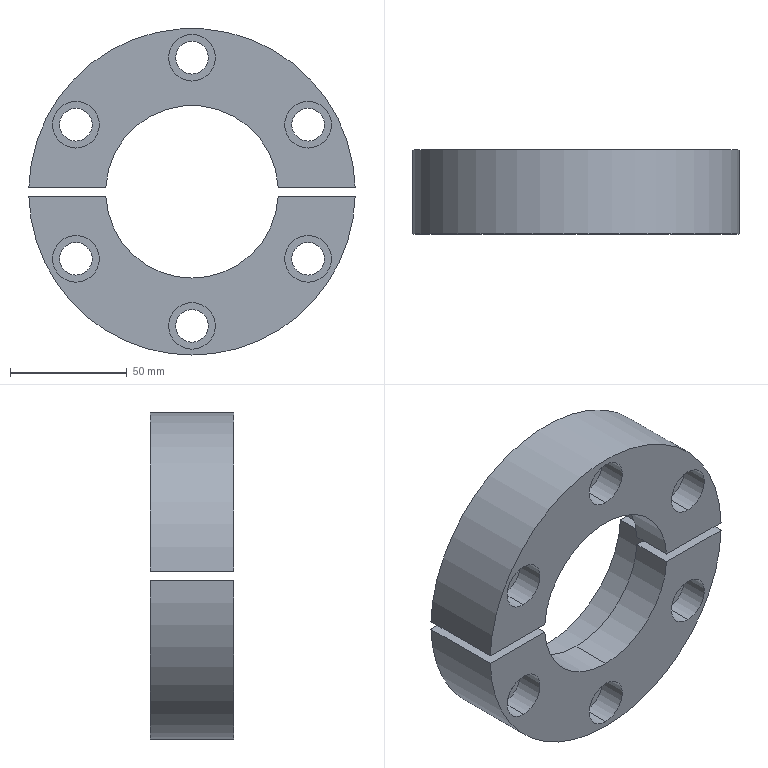Part | STEP file | OP10-029_setting flange | 2 solids | 49 faces | box 139.943 x 36 x 140 mm | volume 309110 mm3 | cylinder 33 | plane 16 | commonest cylinder face diameters 14 x12 20 x12 74 x3 90 x3 140 x3